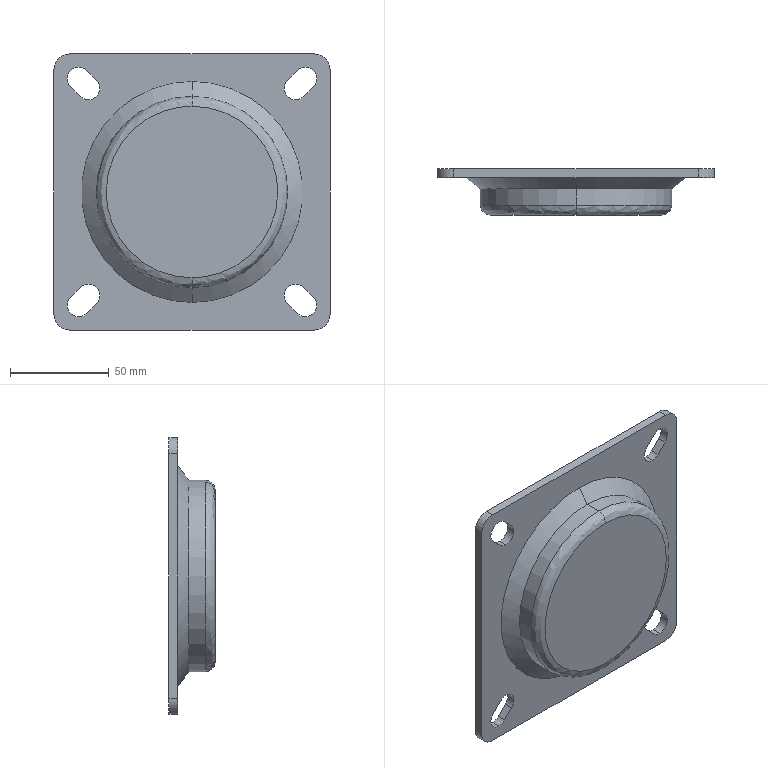Part | STEP file | CDAN75-Ms | 1 solid | 40 faces | box 140 x 23.5 x 140 mm | volume 226200 mm3 | cylinder 20 | plane 16 | spline 2 | cone 2 | commonest cylinder face diameters 11.5 x12 16 x4 72 x2 97 x2